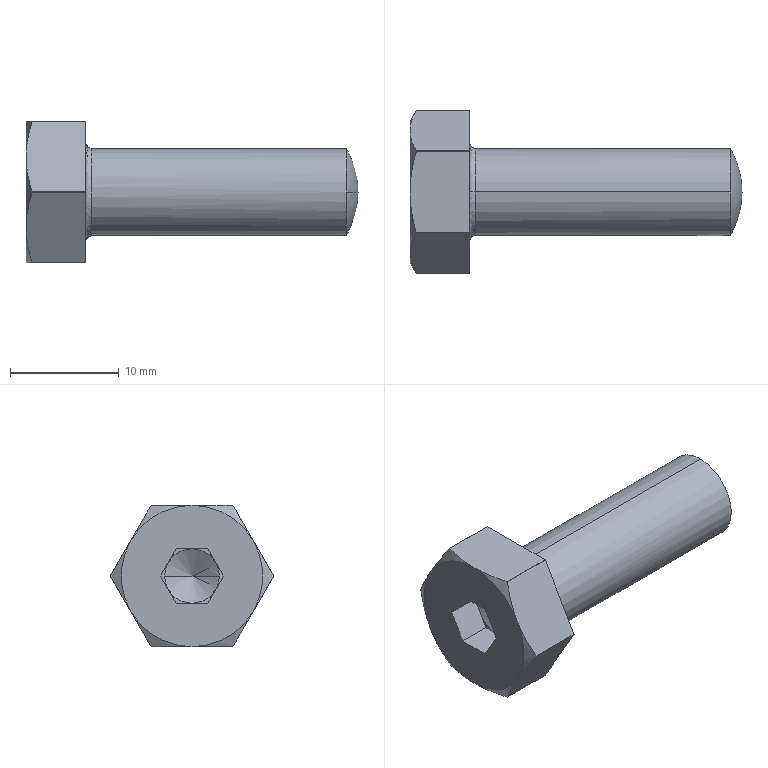Part | STEP file | Sceond1_7 | 1 solid | 40 faces | box 30.5 x 15 x 13 mm | volume 1960 mm3 | plane 20 | cylinder 8 | cone 8 | spline 4 | commonest cylinder face diameters 15 x6 8 x2